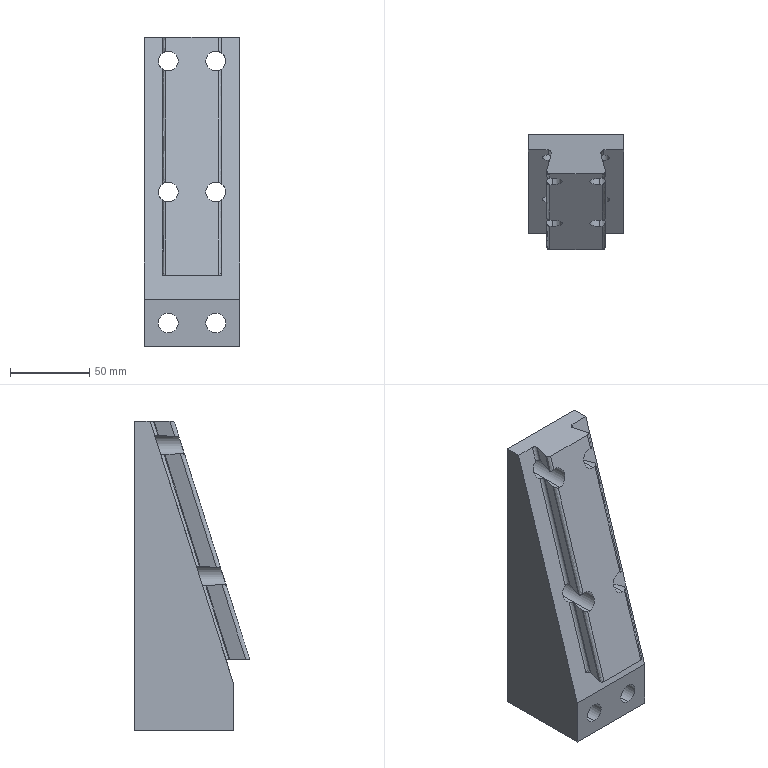Part | SolidWorks | features BaseBody 1 | 1 solid | 45 faces | box 60 x 72.691 x 195 mm | volume 513448 mm3 | spline 18 | plane 15 | cylinder 12 | commonest cylinder face diameters 12.5 x12